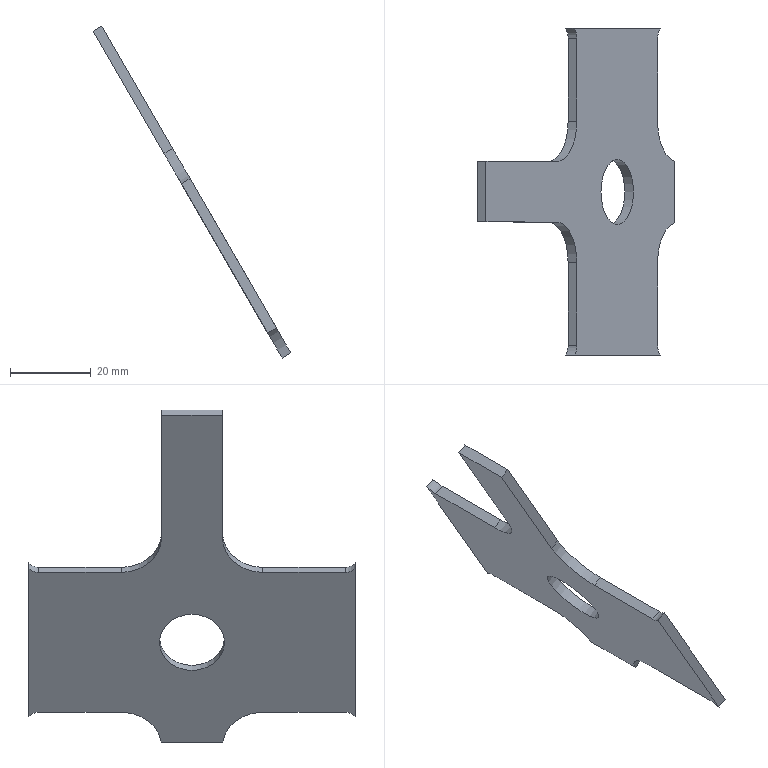Part | STEP file | lll_id4622_x_t | 1 solid | 21 faces | box 48.915 x 81 x 82.223 mm | volume 9822 mm3 | plane 12 | cylinder 9 | commonest cylinder face diameters 6 x4 20 x4 16.1 x1
STEP:
#1=CARTESIAN_POINT('',(3818.5,38.,-151.471));
#2=VERTEX_POINT('',#1);
#3=CARTESIAN_POINT('',(3818.5,17.5,-151.471));
#4=VERTEX_POINT('',#3);
#5=CARTESIAN_POINT('',(3818.5,38.,-151.471));
#6=DIRECTION('',(0.,-1.,0.));
#7=VECTOR('',#6,1.);
#8=LINE('',#5,#7);
#9=EDGE_CURVE('',#2,#4,#8,.T.);
#10=ORIENTED_EDGE('',*,*,#9,.T.);
#11=CARTESIAN_POINT('',(3820.665,17.5,-150.221));
#12=VERTEX_POINT('',#11);
#13=CARTESIAN_POINT('',(3820.665,17.5,-150.221));
#14=DIRECTION('',(0.866,0.,0.5));
#15=VECTOR('',#14,1.);
#16=LINE('',#13,#15);
#17=EDGE_CURVE('',#4,#12,#16,.T.);
#18=ORIENTED_EDGE('',*,*,#17,.T.);
#19=CARTESIAN_POINT('',(3820.665,38.,-150.221));
#20=VERTEX_POINT('',#19);
#21=CARTESIAN_POINT('',(3820.665,38.,-150.221));
#22=DIRECTION('',(0.,-1.,0.));
#23=VECTOR('',#22,1.);
#24=LINE('',#21,#23);
#25=EDGE_CURVE('',#20,#12,#24,.T.);
#26=ORIENTED_EDGE('',*,*,#25,.F.);
#27=CARTESIAN_POINT('',(3820.665,38.,-150.221));
#28=DIRECTION('',(0.866,0.,0.5));
#29=VECTOR('',#28,1.);
#30=LINE('',#27,#29);
#31=EDGE_CURVE('',#2,#20,#30,.T.);
#32=ORIENTED_EDGE('',*,*,#31,.F.);
#33=EDGE_LOOP('',(#10,#18,#26,#32));
#34=FACE_OUTER_BOUND('',#33,.T.);
#35=CARTESIAN_POINT('',(3820.665,38.,-150.221));
#36=DIRECTION('',(0.5,0.,-0.866));
#37=DIRECTION('',(-0.866,0.,-0.5));
#38=AXIS2_PLACEMENT_3D('',#35,#36,#37);
#39=PLANE('',#38);
#40=ADVANCED_FACE('',(#34),#39,.F.);
#41=CARTESIAN_POINT('',(3819.994,40.5,-149.059));
#42=VERTEX_POINT('',#41);
#43=CARTESIAN_POINT('',(3819.165,38.,-147.623));
#44=DIRECTION('',(-0.866,0.,-0.5));
#45=DIRECTION('',(-0.5,0.,0.866));
#46=AXIS2_PLACEMENT_3D('',#43,#44,#45);
#47=CIRCLE('',#46,3.);
#48=EDGE_CURVE('',#42,#20,#47,.T.);
#49=ORIENTED_EDGE('',*,*,#48,.F.);
#50=CARTESIAN_POINT('',(3817.829,40.5,-150.309));
#51=VERTEX_POINT('',#50);
#52=CARTESIAN_POINT('',(3818.912,40.5,-149.684));
#53=DIRECTION('',(-0.866,0.000000008,-0.5));
#54=VECTOR('',#53,1.);
#55=LINE('',#52,#54);
#56=EDGE_CURVE('',#42,#51,#55,.T.);
#57=ORIENTED_EDGE('',*,*,#56,.T.);
#58=CARTESIAN_POINT('',(3817.,38.,-148.873));
#59=DIRECTION('',(-0.866,0.,-0.5));
#60=DIRECTION('',(-0.5,0.,0.866));
#61=AXIS2_PLACEMENT_3D('',#58,#59,#60);
#62=CIRCLE('',#61,3.);
#63=EDGE_CURVE('',#51,#2,#62,.T.);
#64=ORIENTED_EDGE('',*,*,#63,.T.);
#65=ORIENTED_EDGE('',*,*,#31,.T.);
#66=EDGE_LOOP('',(#49,#57,#64,#65));
#67=FACE_OUTER_BOUND('',#66,.T.);
#68=CARTESIAN_POINT('',(3819.165,38.,-147.623));
#69=DIRECTION('',(-0.866,0.,-0.5));
#70=DIRECTION('',(-0.5,0.,0.866));
#71=AXIS2_PLACEMENT_3D('',#68,#69,#70);
#72=CYLINDRICAL_SURFACE('',#71,3.);
#73=ADVANCED_FACE('',(#67),#72,.F.);
#74=CARTESIAN_POINT('',(3841.336,40.5,-186.024));
#75=VERTEX_POINT('',#74);
#76=CARTESIAN_POINT('',(3839.171,40.5,-187.274));
#77=VERTEX_POINT('',#76);
#78=CARTESIAN_POINT('',(3840.253,40.5,-186.649));
#79=DIRECTION('',(-0.866,0.000000008,-0.5));
#80=VECTOR('',#79,1.);
#81=LINE('',#78,#80);
#82=EDGE_CURVE('',#75,#77,#81,.T.);
#83=ORIENTED_EDGE('',*,*,#82,.T.);
#84=CARTESIAN_POINT('',(9079.441,40.5,-9263.689));
#85=DIRECTION('',(-0.5,0.,0.866));
#86=VECTOR('',#85,1.);
#87=LINE('',#84,#86);
#88=EDGE_CURVE('',#77,#51,#87,.T.);
#89=ORIENTED_EDGE('',*,*,#88,.T.);
#90=ORIENTED_EDGE('',*,*,#56,.F.);
#91=CARTESIAN_POINT('',(9081.607,40.5,-9262.439));
#92=DIRECTION('',(0.5,0.,-0.866));
#93=VECTOR('',#92,1.);
#94=LINE('',#91,#93);
#95=EDGE_CURVE('',#42,#75,#94,.T.);
#96=ORIENTED_EDGE('',*,*,#95,.T.);
#97=EDGE_LOOP('',(#83,#89,#90,#96));
#98=FACE_OUTER_BOUND('',#97,.T.);
#99=CARTESIAN_POINT('',(3810.878,40.5,-133.27));
#100=DIRECTION('',(-0.000000007,-1.,-0.000000004));
#101=DIRECTION('',(0.866,-0.000000008,0.5));
#102=AXIS2_PLACEMENT_3D('',#99,#100,#101);
#103=PLANE('',#102);
#104=ADVANCED_FACE('',(#98),#103,.F.);
#105=ORIENTED_EDGE('',*,*,#82,.F.);
#106=CARTESIAN_POINT('',(3840.665,38.,-184.862));
#107=VERTEX_POINT('',#106);
#108=CARTESIAN_POINT('',(3842.165,38.,-187.46));
#109=DIRECTION('',(0.866,0.,0.5));
#110=DIRECTION('',(-0.5,0.,0.866));
#111=AXIS2_PLACEMENT_3D('',#108,#109,#110);
#112=CIRCLE('',#111,3.);
#113=EDGE_CURVE('',#75,#107,#112,.T.);
#114=ORIENTED_EDGE('',*,*,#113,.T.);
#115=CARTESIAN_POINT('',(3838.5,38.,-186.112));
#116=VERTEX_POINT('',#115);
#117=CARTESIAN_POINT('',(3840.665,38.,-184.862));
#118=DIRECTION('',(0.866,0.,0.5));
#119=VECTOR('',#118,1.);
#120=LINE('',#117,#119);
#121=EDGE_CURVE('',#116,#107,#120,.T.);
#122=ORIENTED_EDGE('',*,*,#121,.F.);
#123=CARTESIAN_POINT('',(3840.,38.,-188.71));
#124=DIRECTION('',(0.866,0.,0.5));
#125=DIRECTION('',(-0.5,0.,0.866));
#126=AXIS2_PLACEMENT_3D('',#123,#124,#125);
#127=CIRCLE('',#126,3.);
#128=EDGE_CURVE('',#77,#116,#127,.T.);
#129=ORIENTED_EDGE('',*,*,#128,.F.);
#130=EDGE_LOOP('',(#105,#114,#122,#129));
#131=FACE_OUTER_BOUND('',#130,.T.);
#132=CARTESIAN_POINT('',(3842.165,38.,-187.46));
#133=DIRECTION('',(-0.866,0.,-0.5));
#134=DIRECTION('',(-0.5,0.,0.866));
#135=AXIS2_PLACEMENT_3D('',#132,#133,#134);
#136=CYLINDRICAL_SURFACE('',#135,3.);
#137=ADVANCED_FACE('',(#131),#136,.F.);
#138=CARTESIAN_POINT('',(3838.5,17.5,-186.112));
#139=VERTEX_POINT('',#138);
#140=CARTESIAN_POINT('',(3838.5,38.,-186.112));
#141=DIRECTION('',(0.,-1.,0.));
#142=VECTOR('',#141,1.);
#143=LINE('',#140,#142);
#144=EDGE_CURVE('',#116,#139,#143,.T.);
#145=ORIENTED_EDGE('',*,*,#144,.F.);
#146=ORIENTED_EDGE('',*,*,#121,.T.);
#147=CARTESIAN_POINT('',(3840.665,17.5,-184.862));
#148=VERTEX_POINT('',#147);
#149=CARTESIAN_POINT('',(3840.665,38.,-184.862));
#150=DIRECTION('',(0.,-1.,0.));
#151=VECTOR('',#150,1.);
#152=LINE('',#149,#151);
#153=EDGE_CURVE('',#107,#148,#152,.T.);
#154=ORIENTED_EDGE('',*,*,#153,.T.);
#155=CARTESIAN_POINT('',(3840.665,17.5,-184.862));
#156=DIRECTION('',(0.866,0.,0.5));
#157=VECTOR('',#156,1.);
#158=LINE('',#155,#157);
#159=EDGE_CURVE('',#139,#148,#158,.T.);
#160=ORIENTED_EDGE('',*,*,#159,.F.);
#161=EDGE_LOOP('',(#145,#146,#154,#160));
#162=FACE_OUTER_BOUND('',#161,.T.);
#163=CARTESIAN_POINT('',(3840.665,38.,-184.862));
#164=DIRECTION('',(0.5,0.,-0.866));
#165=DIRECTION('',(-0.866,0.,-0.5));
#166=AXIS2_PLACEMENT_3D('',#163,#164,#165);
#167=PLANE('',#166);
#168=ADVANCED_FACE('',(#162),#167,.T.);
#169=CARTESIAN_POINT('',(3844.915,7.613,-192.223));
#170=VERTEX_POINT('',#169);
#171=CARTESIAN_POINT('',(3845.665,17.5,-193.522));
#172=DIRECTION('',(0.866,0.,0.5));
#173=DIRECTION('',(-0.5,0.,0.866));
#174=AXIS2_PLACEMENT_3D('',#171,#172,#173);
#175=CIRCLE('',#174,10.);
#176=EDGE_CURVE('',#148,#170,#175,.T.);
#177=ORIENTED_EDGE('',*,*,#176,.T.);
#178=CARTESIAN_POINT('',(3842.75,7.613,-193.473));
#179=VERTEX_POINT('',#178);
#180=CARTESIAN_POINT('',(3844.915,7.613,-192.223));
#181=DIRECTION('',(0.866,0.,0.5));
#182=VECTOR('',#181,1.);
#183=LINE('',#180,#182);
#184=EDGE_CURVE('',#179,#170,#183,.T.);
#185=ORIENTED_EDGE('',*,*,#184,.F.);
#186=CARTESIAN_POINT('',(3843.5,17.5,-194.772));
#187=DIRECTION('',(0.866,0.,0.5));
#188=DIRECTION('',(-0.5,0.,0.866));
#189=AXIS2_PLACEMENT_3D('',#186,#187,#188);
#190=CIRCLE('',#189,10.);
#191=EDGE_CURVE('',#139,#179,#190,.T.);
#192=ORIENTED_EDGE('',*,*,#191,.F.);
#193=ORIENTED_EDGE('',*,*,#159,.T.);
#194=EDGE_LOOP('',(#177,#185,#192,#193));
#195=FACE_OUTER_BOUND('',#194,.T.);
#196=CARTESIAN_POINT('',(3845.665,17.5,-193.522));
#197=DIRECTION('',(-0.866,0.,-0.5));
#198=DIRECTION('',(-0.5,0.,0.866));
#199=AXIS2_PLACEMENT_3D('',#196,#197,#198);
#200=CYLINDRICAL_SURFACE('',#199,10.);
#201=ADVANCED_FACE('',(#195),#200,.F.);
#202=CARTESIAN_POINT('',(3842.75,-7.613,-193.473));
#203=VERTEX_POINT('',#202);
#204=CARTESIAN_POINT('',(3838.5,-17.5,-186.112));
#205=VERTEX_POINT('',#204);
#206=CARTESIAN_POINT('',(3843.5,-17.5,-194.772));
#207=DIRECTION('',(0.866,0.,0.5));
#208=DIRECTION('',(-0.5,0.,0.866));
#209=AXIS2_PLACEMENT_3D('',#206,#207,#208);
#210=CIRCLE('',#209,10.);
#211=EDGE_CURVE('',#203,#205,#210,.T.);
#212=ORIENTED_EDGE('',*,*,#211,.F.);
#213=CARTESIAN_POINT('',(3844.915,-7.613,-192.223));
#214=VERTEX_POINT('',#213);
#215=CARTESIAN_POINT('',(3844.915,-7.613,-192.223));
#216=DIRECTION('',(-0.866,0.,-0.5));
#217=VECTOR('',#216,1.);
#218=LINE('',#215,#217);
#219=EDGE_CURVE('',#214,#203,#218,.T.);
#220=ORIENTED_EDGE('',*,*,#219,.F.);
#221=CARTESIAN_POINT('',(3840.665,-17.5,-184.862));
#222=VERTEX_POINT('',#221);
#223=CARTESIAN_POINT('',(3845.665,-17.5,-193.522));
#224=DIRECTION('',(0.866,0.,0.5));
#225=DIRECTION('',(-0.5,0.,0.866));
#226=AXIS2_PLACEMENT_3D('',#223,#224,#225);
#227=CIRCLE('',#226,10.);
#228=EDGE_CURVE('',#214,#222,#227,.T.);
#229=ORIENTED_EDGE('',*,*,#228,.T.);
#230=CARTESIAN_POINT('',(3840.665,-17.5,-184.862));
#231=DIRECTION('',(0.866,0.,0.5));
#232=VECTOR('',#231,1.);
#233=LINE('',#230,#232);
#234=EDGE_CURVE('',#205,#222,#233,.T.);
#235=ORIENTED_EDGE('',*,*,#234,.F.);
#236=EDGE_LOOP('',(#212,#220,#229,#235));
#237=FACE_OUTER_BOUND('',#236,.T.);
#238=CARTESIAN_POINT('',(3845.665,-17.5,-193.522));
#239=DIRECTION('',(-0.866,0.,-0.5));
#240=DIRECTION('',(-0.5,0.,0.866));
#241=AXIS2_PLACEMENT_3D('',#238,#239,#240);
#242=CYLINDRICAL_SURFACE('',#241,10.);
#243=ADVANCED_FACE('',(#237),#242,.F.);
#244=CARTESIAN_POINT('',(3838.5,-38.,-186.112));
#245=VERTEX_POINT('',#244);
#246=CARTESIAN_POINT('',(3838.5,-17.5,-186.112));
#247=DIRECTION('',(0.,-1.,0.));
#248=VECTOR('',#247,1.);
#249=LINE('',#246,#248);
#250=EDGE_CURVE('',#205,#245,#249,.T.);
#251=ORIENTED_EDGE('',*,*,#250,.F.);
#252=ORIENTED_EDGE('',*,*,#234,.T.);
#253=CARTESIAN_POINT('',(3840.665,-38.,-184.862));
#254=VERTEX_POINT('',#253);
#255=CARTESIAN_POINT('',(3840.665,-17.5,-184.862));
#256=DIRECTION('',(0.,-1.,0.));
#257=VECTOR('',#256,1.);
#258=LINE('',#255,#257);
#259=EDGE_CURVE('',#222,#254,#258,.T.);
#260=ORIENTED_EDGE('',*,*,#259,.T.);
#261=CARTESIAN_POINT('',(3840.665,-38.,-184.862));
#262=DIRECTION('',(0.866,0.,0.5));
#263=VECTOR('',#262,1.);
#264=LINE('',#261,#263);
#265=EDGE_CURVE('',#245,#254,#264,.T.);
#266=ORIENTED_EDGE('',*,*,#265,.F.);
#267=EDGE_LOOP('',(#251,#252,#260,#266));
#268=FACE_OUTER_BOUND('',#267,.T.);
#269=CARTESIAN_POINT('',(3840.665,-17.5,-184.862));
#270=DIRECTION('',(0.5,0.,-0.866));
#271=DIRECTION('',(-0.866,0.,-0.5));
#272=AXIS2_PLACEMENT_3D('',#269,#270,#271);
#273=PLANE('',#272);
#274=ADVANCED_FACE('',(#268),#273,.T.);
#275=CARTESIAN_POINT('',(3841.336,-40.5,-186.024));
#276=VERTEX_POINT('',#275);
#277=CARTESIAN_POINT('',(3839.171,-40.5,-187.274));
#278=VERTEX_POINT('',#277);
#279=CARTESIAN_POINT('',(3841.336,-40.5,-186.024));
#280=DIRECTION('',(-0.866,0.,-0.5));
#281=VECTOR('',#280,1.);
#282=LINE('',#279,#281);
#283=EDGE_CURVE('',#276,#278,#282,.T.);
#284=ORIENTED_EDGE('',*,*,#283,.T.);
#285=CARTESIAN_POINT('',(3840.,-38.,-188.71));
#286=DIRECTION('',(0.866,0.,0.5));
#287=DIRECTION('',(-0.5,0.,0.866));
#288=AXIS2_PLACEMENT_3D('',#285,#286,#287);
#289=CIRCLE('',#288,3.);
#290=EDGE_CURVE('',#245,#278,#289,.T.);
#291=ORIENTED_EDGE('',*,*,#290,.F.);
#292=ORIENTED_EDGE('',*,*,#265,.T.);
#293=CARTESIAN_POINT('',(3842.165,-38.,-187.46));
#294=DIRECTION('',(0.866,0.,0.5));
#295=DIRECTION('',(-0.5,0.,0.866));
#296=AXIS2_PLACEMENT_3D('',#293,#294,#295);
#297=CIRCLE('',#296,3.);
#298=EDGE_CURVE('',#254,#276,#297,.T.);
#299=ORIENTED_EDGE('',*,*,#298,.T.);
#300=EDGE_LOOP('',(#284,#291,#292,#299));
#301=FACE_OUTER_BOUND('',#300,.T.);
#302=CARTESIAN_POINT('',(3842.165,-38.,-187.46));
#303=DIRECTION('',(-0.866,0.,-0.5));
#304=DIRECTION('',(-0.5,0.,0.866));
#305=AXIS2_PLACEMENT_3D('',#302,#303,#304);
#306=CYLINDRICAL_SURFACE('',#305,3.);
#307=ADVANCED_FACE('',(#301),#306,.F.);
#308=ORIENTED_EDGE('',*,*,#283,.F.);
#309=CARTESIAN_POINT('',(3819.994,-40.5,-149.059));
#310=VERTEX_POINT('',#309);
#311=CARTESIAN_POINT('',(9081.607,-40.5,-9262.439));
#312=DIRECTION('',(0.5,0.,-0.866));
#313=VECTOR('',#312,1.);
#314=LINE('',#311,#313);
#315=EDGE_CURVE('',#310,#276,#314,.T.);
#316=ORIENTED_EDGE('',*,*,#315,.F.);
#317=CARTESIAN_POINT('',(3817.829,-40.5,-150.309));
#318=VERTEX_POINT('',#317);
#319=CARTESIAN_POINT('',(3819.994,-40.5,-149.059));
#320=DIRECTION('',(0.866,0.,0.5));
#321=VECTOR('',#320,1.);
#322=LINE('',#319,#321);
#323=EDGE_CURVE('',#318,#310,#322,.T.);
#324=ORIENTED_EDGE('',*,*,#323,.F.);
#325=CARTESIAN_POINT('',(9079.441,-40.5,-9263.689));
#326=DIRECTION('',(0.5,0.,-0.866));
#327=VECTOR('',#326,1.);
#328=LINE('',#325,#327);
#329=EDGE_CURVE('',#318,#278,#328,.T.);
#330=ORIENTED_EDGE('',*,*,#329,.T.);
#331=EDGE_LOOP('',(#308,#316,#324,#330));
#332=FACE_OUTER_BOUND('',#331,.T.);
#333=CARTESIAN_POINT('',(3808.713,-40.5,-134.52));
#334=DIRECTION('',(0.,1.,0.));
#335=DIRECTION('',(-0.866,0.,-0.5));
#336=AXIS2_PLACEMENT_3D('',#333,#334,#335);
#337=PLANE('',#336);
#338=ADVANCED_FACE('',(#332),#337,.F.);
#339=ORIENTED_EDGE('',*,*,#323,.T.);
#340=CARTESIAN_POINT('',(3820.665,-38.,-150.221));
#341=VERTEX_POINT('',#340);
#342=CARTESIAN_POINT('',(3819.165,-38.,-147.623));
#343=DIRECTION('',(0.866,0.,0.5));
#344=DIRECTION('',(-0.5,0.,0.866));
#345=AXIS2_PLACEMENT_3D('',#342,#343,#344);
#346=CIRCLE('',#345,3.);
#347=EDGE_CURVE('',#310,#341,#346,.T.);
#348=ORIENTED_EDGE('',*,*,#347,.T.);
#349=CARTESIAN_POINT('',(3818.5,-38.,-151.471));
#350=VERTEX_POINT('',#349);
#351=CARTESIAN_POINT('',(3820.665,-38.,-150.221));
#352=DIRECTION('',(0.866,0.,0.5));
#353=VECTOR('',#352,1.);
#354=LINE('',#351,#353);
#355=EDGE_CURVE('',#350,#341,#354,.T.);
#356=ORIENTED_EDGE('',*,*,#355,.F.);
#357=CARTESIAN_POINT('',(3817.,-38.,-148.873));
#358=DIRECTION('',(0.866,0.,0.5));
#359=DIRECTION('',(-0.5,0.,0.866));
#360=AXIS2_PLACEMENT_3D('',#357,#358,#359);
#361=CIRCLE('',#360,3.);
#362=EDGE_CURVE('',#318,#350,#361,.T.);
#363=ORIENTED_EDGE('',*,*,#362,.F.);
#364=EDGE_LOOP('',(#339,#348,#356,#363));
#365=FACE_OUTER_BOUND('',#364,.T.);
#366=CARTESIAN_POINT('',(3819.165,-38.,-147.623));
#367=DIRECTION('',(-0.866,0.,-0.5));
#368=DIRECTION('',(-0.5,0.,0.866));
#369=AXIS2_PLACEMENT_3D('',#366,#367,#368);
#370=CYLINDRICAL_SURFACE('',#369,3.);
#371=ADVANCED_FACE('',(#365),#370,.F.);
#372=CARTESIAN_POINT('',(3818.5,-17.5,-151.471));
#373=VERTEX_POINT('',#372);
#374=CARTESIAN_POINT('',(3818.5,-38.,-151.471));
#375=DIRECTION('',(0.,1.,0.));
#376=VECTOR('',#375,1.);
#377=LINE('',#374,#376);
#378=EDGE_CURVE('',#350,#373,#377,.T.);
#379=ORIENTED_EDGE('',*,*,#378,.F.);
#380=ORIENTED_EDGE('',*,*,#355,.T.);
#381=CARTESIAN_POINT('',(3820.665,-17.5,-150.221));
#382=VERTEX_POINT('',#381);
#383=CARTESIAN_POINT('',(3820.665,-38.,-150.221));
#384=DIRECTION('',(0.,1.,0.));
#385=VECTOR('',#384,1.);
#386=LINE('',#383,#385);
#387=EDGE_CURVE('',#341,#382,#386,.T.);
#388=ORIENTED_EDGE('',*,*,#387,.T.);
#389=CARTESIAN_POINT('',(3820.665,-17.5,-150.221));
#390=DIRECTION('',(0.866,0.,0.5));
#391=VECTOR('',#390,1.);
#392=LINE('',#389,#391);
#393=EDGE_CURVE('',#373,#382,#392,.T.);
#394=ORIENTED_EDGE('',*,*,#393,.F.);
#395=EDGE_LOOP('',(#379,#380,#388,#394));
#396=FACE_OUTER_BOUND('',#395,.T.);
#397=CARTESIAN_POINT('',(3820.665,-38.,-150.221));
#398=DIRECTION('',(-0.5,0.,0.866));
#399=DIRECTION('',(0.,1.,0.));
#400=AXIS2_PLACEMENT_3D('',#397,#398,#399);
#401=PLANE('',#400);
#402=ADVANCED_FACE('',(#396),#401,.T.);
#403=CARTESIAN_POINT('',(3826.64,0.,-160.57));
#404=VERTEX_POINT('',#403);
#405=CARTESIAN_POINT('',(3830.665,0.,-167.542));
#406=DIRECTION('',(0.866,0.,0.5));
#407=DIRECTION('',(-0.5,0.,0.866));
#408=AXIS2_PLACEMENT_3D('',#405,#406,#407);
#409=CIRCLE('',#408,8.05);
#410=EDGE_CURVE('',#404,#404,#409,.T.);
#411=ORIENTED_EDGE('',*,*,#410,.T.);
#412=EDGE_LOOP('',(#411));
#413=FACE_BOUND('',#412,.T.);
#414=CARTESIAN_POINT('',(3824.475,0.,-161.82));
#415=VERTEX_POINT('',#414);
#416=CARTESIAN_POINT('',(3828.5,0.,-168.792));
#417=DIRECTION('',(0.866,0.,0.5));
#418=DIRECTION('',(-0.5,0.,0.866));
#419=AXIS2_PLACEMENT_3D('',#416,#417,#418);
#420=CIRCLE('',#419,8.05);
#421=EDGE_CURVE('',#415,#415,#420,.T.);
#422=ORIENTED_EDGE('',*,*,#421,.F.);
#423=EDGE_LOOP('',(#422));
#424=FACE_BOUND('',#423,.T.);
#425=CARTESIAN_POINT('',(3830.665,0.,-167.542));
#426=DIRECTION('',(-0.866,0.,-0.5));
#427=DIRECTION('',(-0.5,0.,0.866));
#428=AXIS2_PLACEMENT_3D('',#425,#426,#427);
#429=CYLINDRICAL_SURFACE('',#428,8.05);
#430=ADVANCED_FACE('',(#413,#424),#429,.F.);
#431=CARTESIAN_POINT('',(3813.5,-7.5,-142.811));
#432=VERTEX_POINT('',#431);
#433=CARTESIAN_POINT('',(3813.5,-17.5,-142.811));
#434=DIRECTION('',(0.866,0.,0.5));
#435=DIRECTION('',(-0.5,0.,0.866));
#436=AXIS2_PLACEMENT_3D('',#433,#434,#435);
#437=CIRCLE('',#436,10.);
#438=EDGE_CURVE('',#373,#432,#437,.T.);
#439=ORIENTED_EDGE('',*,*,#438,.F.);
#440=ORIENTED_EDGE('',*,*,#393,.T.);
#441=CARTESIAN_POINT('',(3815.665,-7.5,-141.561));
#442=VERTEX_POINT('',#441);
#443=CARTESIAN_POINT('',(3815.665,-17.5,-141.561));
#444=DIRECTION('',(0.866,0.,0.5));
#445=DIRECTION('',(-0.5,0.,0.866));
#446=AXIS2_PLACEMENT_3D('',#443,#444,#445);
#447=CIRCLE('',#446,10.);
#448=EDGE_CURVE('',#382,#442,#447,.T.);
#449=ORIENTED_EDGE('',*,*,#448,.T.);
#450=CARTESIAN_POINT('',(3815.665,-7.5,-141.561));
#451=DIRECTION('',(0.866,0.,0.5));
#452=VECTOR('',#451,1.);
#453=LINE('',#450,#452);
#454=EDGE_CURVE('',#432,#442,#453,.T.);
#455=ORIENTED_EDGE('',*,*,#454,.F.);
#456=EDGE_LOOP('',(#439,#440,#449,#455));
#457=FACE_OUTER_BOUND('',#456,.T.);
#458=CARTESIAN_POINT('',(3815.665,-17.5,-141.561));
#459=DIRECTION('',(-0.866,0.,-0.5));
#460=DIRECTION('',(-0.5,0.,0.866));
#461=AXIS2_PLACEMENT_3D('',#458,#459,#460);
#462=CYLINDRICAL_SURFACE('',#461,10.);
#463=ADVANCED_FACE('',(#457),#462,.F.);
#464=CARTESIAN_POINT('',(3813.5,7.5,-142.811));
#465=VERTEX_POINT('',#464);
#466=CARTESIAN_POINT('',(3813.5,17.5,-142.811));
#467=DIRECTION('',(-0.866,0.,-0.5));
#468=DIRECTION('',(-0.5,0.,0.866));
#469=AXIS2_PLACEMENT_3D('',#466,#467,#468);
#470=CIRCLE('',#469,10.);
#471=EDGE_CURVE('',#4,#465,#470,.T.);
#472=ORIENTED_EDGE('',*,*,#471,.T.);
#473=CARTESIAN_POINT('',(3815.665,7.5,-141.561));
#474=VERTEX_POINT('',#473);
#475=CARTESIAN_POINT('',(3815.665,7.5,-141.561));
#476=DIRECTION('',(0.866,0.,0.5));
#477=VECTOR('',#476,1.);
#478=LINE('',#475,#477);
#479=EDGE_CURVE('',#465,#474,#478,.T.);
#480=ORIENTED_EDGE('',*,*,#479,.T.);
#481=CARTESIAN_POINT('',(3815.665,17.5,-141.561));
#482=DIRECTION('',(-0.866,0.,-0.5));
#483=DIRECTION('',(-0.5,0.,0.866));
#484=AXIS2_PLACEMENT_3D('',#481,#482,#483);
#485=CIRCLE('',#484,10.);
#486=EDGE_CURVE('',#12,#474,#485,.T.);
#487=ORIENTED_EDGE('',*,*,#486,.F.);
#488=ORIENTED_EDGE('',*,*,#17,.F.);
#489=EDGE_LOOP('',(#472,#480,#487,#488));
#490=FACE_OUTER_BOUND('',#489,.T.);
#491=CARTESIAN_POINT('',(3815.665,17.5,-141.561));
#492=DIRECTION('',(-0.866,0.,-0.5));
#493=DIRECTION('',(-0.5,0.,0.866));
#494=AXIS2_PLACEMENT_3D('',#491,#492,#493);
#495=CYLINDRICAL_SURFACE('',#494,10.);
#496=ADVANCED_FACE('',(#490),#495,.F.);
#497=CARTESIAN_POINT('',(3798.165,-7.5,-111.25));
#498=VERTEX_POINT('',#497);
#499=CARTESIAN_POINT('',(3796.,-7.5,-112.5));
#500=VERTEX_POINT('',#499);
#501=CARTESIAN_POINT('',(3798.165,-7.5,-111.25));
#502=DIRECTION('',(-0.866,0.,-0.5));
#503=VECTOR('',#502,1.);
#504=LINE('',#501,#503);
#505=EDGE_CURVE('',#498,#500,#504,.T.);
#506=ORIENTED_EDGE('',*,*,#505,.T.);
#507=CARTESIAN_POINT('',(3813.5,-7.5,-142.811));
#508=DIRECTION('',(-0.5,0.,0.866));
#509=VECTOR('',#508,1.);
#510=LINE('',#507,#509);
#511=EDGE_CURVE('',#432,#500,#510,.T.);
#512=ORIENTED_EDGE('',*,*,#511,.F.);
#513=ORIENTED_EDGE('',*,*,#454,.T.);
#514=CARTESIAN_POINT('',(3815.665,-7.5,-141.561));
#515=DIRECTION('',(-0.5,0.,0.866));
#516=VECTOR('',#515,1.);
#517=LINE('',#514,#516);
#518=EDGE_CURVE('',#442,#498,#517,.T.);
#519=ORIENTED_EDGE('',*,*,#518,.T.);
#520=EDGE_LOOP('',(#506,#512,#513,#519));
#521=FACE_OUTER_BOUND('',#520,.T.);
#522=CARTESIAN_POINT('',(3815.665,-7.5,-141.561));
#523=DIRECTION('',(0.,-1.,0.));
#524=DIRECTION('',(-0.5,0.,0.866));
#525=AXIS2_PLACEMENT_3D('',#522,#523,#524);
#526=PLANE('',#525);
#527=ADVANCED_FACE('',(#521),#526,.T.);
#528=CARTESIAN_POINT('',(3796.,7.5,-112.5));
#529=VERTEX_POINT('',#528);
#530=CARTESIAN_POINT('',(3813.5,7.5,-142.811));
#531=DIRECTION('',(-0.5,0.,0.866));
#532=VECTOR('',#531,1.);
#533=LINE('',#530,#532);
#534=EDGE_CURVE('',#465,#529,#533,.T.);
#535=ORIENTED_EDGE('',*,*,#534,.T.);
#536=CARTESIAN_POINT('',(3798.165,7.5,-111.25));
#537=VERTEX_POINT('',#536);
#538=CARTESIAN_POINT('',(3798.165,7.5,-111.25));
#539=DIRECTION('',(0.866,0.,0.5));
#540=VECTOR('',#539,1.);
#541=LINE('',#538,#540);
#542=EDGE_CURVE('',#529,#537,#541,.T.);
#543=ORIENTED_EDGE('',*,*,#542,.T.);
#544=CARTESIAN_POINT('',(3815.665,7.5,-141.561));
#545=DIRECTION('',(-0.5,0.,0.866));
#546=VECTOR('',#545,1.);
#547=LINE('',#544,#546);
#548=EDGE_CURVE('',#474,#537,#547,.T.);
#549=ORIENTED_EDGE('',*,*,#548,.F.);
#550=ORIENTED_EDGE('',*,*,#479,.F.);
#551=EDGE_LOOP('',(#535,#543,#549,#550));
#552=FACE_OUTER_BOUND('',#551,.T.);
#553=CARTESIAN_POINT('',(3815.665,7.5,-141.561));
#554=DIRECTION('',(0.,-1.,0.));
#555=DIRECTION('',(-0.5,0.,0.866));
#556=AXIS2_PLACEMENT_3D('',#553,#554,#555);
#557=PLANE('',#556);
#558=ADVANCED_FACE('',(#552),#557,.F.);
#559=ORIENTED_EDGE('',*,*,#410,.F.);
#560=EDGE_LOOP('',(#559));
#561=FACE_BOUND('',#560,.T.);
#562=ORIENTED_EDGE('',*,*,#228,.F.);
#563=CARTESIAN_POINT('',(3844.915,-13712.786,-192.223));
#564=DIRECTION('',(0.,-1.,0.));
#565=VECTOR('',#564,1.);
#566=LINE('',#563,#565);
#567=EDGE_CURVE('',#170,#214,#566,.T.);
#568=ORIENTED_EDGE('',*,*,#567,.F.);
#569=ORIENTED_EDGE('',*,*,#176,.F.);
#570=ORIENTED_EDGE('',*,*,#153,.F.);
#571=ORIENTED_EDGE('',*,*,#113,.F.);
#572=ORIENTED_EDGE('',*,*,#95,.F.);
#573=ORIENTED_EDGE('',*,*,#48,.T.);
#574=ORIENTED_EDGE('',*,*,#25,.T.);
#575=ORIENTED_EDGE('',*,*,#486,.T.);
#576=ORIENTED_EDGE('',*,*,#548,.T.);
#577=CARTESIAN_POINT('',(3798.165,-13712.786,-111.25));
#578=DIRECTION('',(0.,1.,0.));
#579=VECTOR('',#578,1.);
#580=LINE('',#577,#579);
#581=EDGE_CURVE('',#498,#537,#580,.T.);
#582=ORIENTED_EDGE('',*,*,#581,.F.);
#583=ORIENTED_EDGE('',*,*,#518,.F.);
#584=ORIENTED_EDGE('',*,*,#448,.F.);
#585=ORIENTED_EDGE('',*,*,#387,.F.);
#586=ORIENTED_EDGE('',*,*,#347,.F.);
#587=ORIENTED_EDGE('',*,*,#315,.T.);
#588=ORIENTED_EDGE('',*,*,#298,.F.);
#589=ORIENTED_EDGE('',*,*,#259,.F.);
#590=EDGE_LOOP('',(#562,#568,#569,#570,#571,#572,#573,#574,#575,#576,#582,#583,#584,#585,#586,#587,#588,#589));
#591=FACE_BOUND('',#590,.T.);
#592=CARTESIAN_POINT('',(9081.607,-13712.786,-9262.439));
#593=DIRECTION('',(-0.866,0.,-0.5));
#594=DIRECTION('',(-0.5,0.,0.866));
#595=AXIS2_PLACEMENT_3D('',#592,#593,#594);
#596=PLANE('',#595);
#597=ADVANCED_FACE('',(#561,#591),#596,.F.);
#598=CARTESIAN_POINT('',(3842.75,-13712.786,-193.473));
#599=DIRECTION('',(0.,1.,0.));
#600=VECTOR('',#599,1.);
#601=LINE('',#598,#600);
#602=EDGE_CURVE('',#203,#179,#601,.T.);
#603=ORIENTED_EDGE('',*,*,#602,.F.);
#604=ORIENTED_EDGE('',*,*,#211,.T.);
#605=ORIENTED_EDGE('',*,*,#250,.T.);
#606=ORIENTED_EDGE('',*,*,#290,.T.);
#607=ORIENTED_EDGE('',*,*,#329,.F.);
#608=ORIENTED_EDGE('',*,*,#362,.T.);
#609=ORIENTED_EDGE('',*,*,#378,.T.);
#610=ORIENTED_EDGE('',*,*,#438,.T.);
#611=ORIENTED_EDGE('',*,*,#511,.T.);
#612=CARTESIAN_POINT('',(3796.,-13712.786,-112.5));
#613=DIRECTION('',(0.,-1.,0.));
#614=VECTOR('',#613,1.);
#615=LINE('',#612,#614);
#616=EDGE_CURVE('',#529,#500,#615,.T.);
#617=ORIENTED_EDGE('',*,*,#616,.F.);
#618=ORIENTED_EDGE('',*,*,#534,.F.);
#619=ORIENTED_EDGE('',*,*,#471,.F.);
#620=ORIENTED_EDGE('',*,*,#9,.F.);
#621=ORIENTED_EDGE('',*,*,#63,.F.);
#622=ORIENTED_EDGE('',*,*,#88,.F.);
#623=ORIENTED_EDGE('',*,*,#128,.T.);
#624=ORIENTED_EDGE('',*,*,#144,.T.);
#625=ORIENTED_EDGE('',*,*,#191,.T.);
#626=EDGE_LOOP('',(#603,#604,#605,#606,#607,#608,#609,#610,#611,#617,#618,#619,#620,#621,#622,#623,#624,#625));
#627=FACE_BOUND('',#626,.T.);
#628=ORIENTED_EDGE('',*,*,#421,.T.);
#629=EDGE_LOOP('',(#628));
#630=FACE_BOUND('',#629,.T.);
#631=CARTESIAN_POINT('',(9079.441,-13712.786,-9263.689));
#632=DIRECTION('',(-0.866,0.,-0.5));
#633=DIRECTION('',(-0.5,0.,0.866));
#634=AXIS2_PLACEMENT_3D('',#631,#632,#633);
#635=PLANE('',#634);
#636=ADVANCED_FACE('',(#627,#630),#635,.T.);
#637=ORIENTED_EDGE('',*,*,#505,.F.);
#638=ORIENTED_EDGE('',*,*,#581,.T.);
#639=ORIENTED_EDGE('',*,*,#542,.F.);
#640=ORIENTED_EDGE('',*,*,#616,.T.);
#641=EDGE_LOOP('',(#637,#638,#639,#640));
#642=FACE_OUTER_BOUND('',#641,.T.);
#643=CARTESIAN_POINT('',(3797.083,0.,-111.875));
#644=DIRECTION('',(0.5,0.,-0.866));
#645=DIRECTION('',(-0.866,0.,-0.5));
#646=AXIS2_PLACEMENT_3D('',#643,#644,#645);
#647=PLANE('',#646);
#648=ADVANCED_FACE('',(#642),#647,.F.);
#649=ORIENTED_EDGE('',*,*,#219,.T.);
#650=ORIENTED_EDGE('',*,*,#602,.T.);
#651=ORIENTED_EDGE('',*,*,#184,.T.);
#652=ORIENTED_EDGE('',*,*,#567,.T.);
#653=EDGE_LOOP('',(#649,#650,#651,#652));
#654=FACE_OUTER_BOUND('',#653,.T.);
#655=CARTESIAN_POINT('',(3827.595,0.000003792,-202.223));
#656=DIRECTION('',(-0.5,0.,0.866));
#657=DIRECTION('',(0.866,0.,0.5));
#658=AXIS2_PLACEMENT_3D('',#655,#656,#657);
#659=PLANE('',#658);
#660=ADVANCED_FACE('',(#654),#659,.F.);
#661=CLOSED_SHELL('',(#40,#73,#104,#137,#168,#201,#243,#274,#307,#338,#371,#402,#430,#463,#496,#527,#558,#597,#636,#648,#660));
#662=MANIFOLD_SOLID_BREP('',#661);
#663=(LENGTH_UNIT()NAMED_UNIT(*)SI_UNIT(.MILLI.,.METRE.));
#664=UNCERTAINTY_MEASURE_WITH_UNIT(LENGTH_MEASURE(0.00002),#663,'','');
#665=(NAMED_UNIT(*)PLANE_ANGLE_UNIT()SI_UNIT($,.RADIAN.));
#666=PLANE_ANGLE_MEASURE_WITH_UNIT(PLANE_ANGLE_MEASURE(0.01745),#665);
#667=DIMENSIONAL_EXPONENTS(0.,0.,0.,0.,0.,0.,0.);
#668=(CONVERSION_BASED_UNIT('DEGREE',#666)NAMED_UNIT(#667)PLANE_ANGLE_UNIT());
#669=(NAMED_UNIT(*)SI_UNIT($,.STERADIAN.)SOLID_ANGLE_UNIT());
#670=(GEOMETRIC_REPRESENTATION_CONTEXT(3)GLOBAL_UNCERTAINTY_ASSIGNED_CONTEXT((#664))GLOBAL_UNIT_ASSIGNED_CONTEXT((#663,#668,#669))REPRESENTATION_CONTEXT('',''));
#671=ADVANCED_BREP_SHAPE_REPRESENTATION('',(#662),#670);